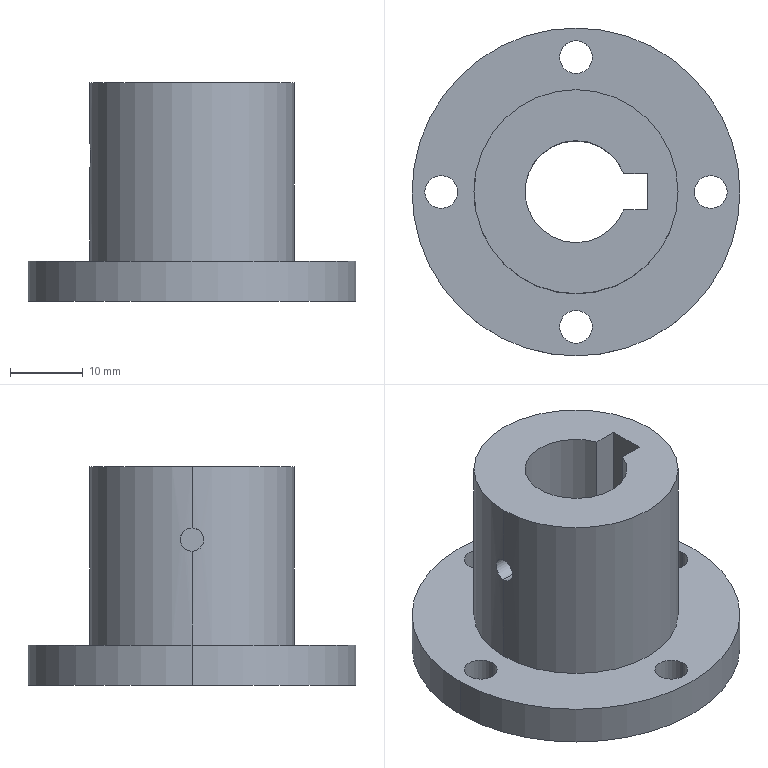Part | STEP file | Coupling | 1 solid | 21 faces | box 45 x 45 x 30 mm | volume 18366 mm3 | cylinder 15 | plane 6 | commonest cylinder face diameters 4.5 x8 3.2 x2 28 x2 45 x2 14 x1
STEP:
#1=CARTESIAN_POINT('',(-14.,0.,21.6));
#2=VERTEX_POINT('',#1);
#3=CARTESIAN_POINT('',(-14.,0.,18.4));
#4=VERTEX_POINT('',#3);
#5=CARTESIAN_POINT('',(-14.,0.,21.6));
#6=CARTESIAN_POINT('',(-14.,-0.1058,21.6));
#7=CARTESIAN_POINT('',(-13.999,-0.2098,21.59));
#8=CARTESIAN_POINT('',(-13.994,-0.4145,21.549));
#9=CARTESIAN_POINT('',(-13.991,-0.5161,21.518));
#10=CARTESIAN_POINT('',(-13.982,-0.7099,21.438));
#11=CARTESIAN_POINT('',(-13.977,-0.8017,21.389));
#12=CARTESIAN_POINT('',(-13.966,-0.9756,21.272));
#13=CARTESIAN_POINT('',(-13.96,-1.058,21.205));
#14=CARTESIAN_POINT('',(-13.942,-1.279,20.984));
#15=CARTESIAN_POINT('',(-13.93,-1.398,20.805));
#16=CARTESIAN_POINT('',(-13.913,-1.558,20.42));
#17=CARTESIAN_POINT('',(-13.908,-1.6,20.209));
#18=CARTESIAN_POINT('',(-13.908,-1.6,19.896));
#19=CARTESIAN_POINT('',(-13.909,-1.59,19.79));
#20=CARTESIAN_POINT('',(-13.914,-1.549,19.585));
#21=CARTESIAN_POINT('',(-13.917,-1.518,19.485));
#22=CARTESIAN_POINT('',(-13.926,-1.438,19.291));
#23=CARTESIAN_POINT('',(-13.931,-1.388,19.198));
#24=CARTESIAN_POINT('',(-13.942,-1.272,19.024));
#25=CARTESIAN_POINT('',(-13.948,-1.206,18.943));
#26=CARTESIAN_POINT('',(-13.96,-1.057,18.794));
#27=CARTESIAN_POINT('',(-13.966,-0.9761,18.728));
#28=CARTESIAN_POINT('',(-13.977,-0.8029,18.612));
#29=CARTESIAN_POINT('',(-13.982,-0.7093,18.562));
#30=CARTESIAN_POINT('',(-13.991,-0.5155,18.482));
#31=CARTESIAN_POINT('',(-13.994,-0.4158,18.451));
#32=CARTESIAN_POINT('',(-13.999,-0.2106,18.41));
#33=CARTESIAN_POINT('',(-14.,-0.1045,18.4));
#34=CARTESIAN_POINT('',(-14.,0.,18.4));
#35=B_SPLINE_CURVE_WITH_KNOTS('',3,(#5,#6,#7,#8,#9,#10,#11,#12,#13,#14,#15,#16,#17,#18,#19,#20,#21,#22,#23,#24,#25,#26,#27,#28,#29,#30,#31,#32,#33,#34),.UNSPECIFIED.,.F.,.F.,(4,2,2,2,2,2,2,2,2,2,2,2,2,2,4),(0.,0.0003129,0.0006258,0.0009387,0.001252,0.001877,0.002503,0.002816,0.003129,0.003442,0.003755,0.004068,0.004381,0.004694,0.005006),.UNSPECIFIED.);
#36=EDGE_CURVE('',#2,#4,#35,.T.);
#37=ORIENTED_EDGE('',*,*,#36,.F.);
#38=CARTESIAN_POINT('',(-7.,0.,21.6));
#39=VERTEX_POINT('',#38);
#40=CARTESIAN_POINT('',(-20.,0.,21.6));
#41=DIRECTION('',(1.,0.,0.));
#42=VECTOR('',#41,1000.);
#43=LINE('',#40,#42);
#44=EDGE_CURVE('',#2,#39,#43,.T.);
#45=ORIENTED_EDGE('',*,*,#44,.T.);
#46=CARTESIAN_POINT('',(-7.,0.,18.4));
#47=VERTEX_POINT('',#46);
#48=CARTESIAN_POINT('',(-7.,0.,18.4));
#49=CARTESIAN_POINT('',(-7.,-0.1061,18.4));
#50=CARTESIAN_POINT('',(-6.998,-0.2103,18.41));
#51=CARTESIAN_POINT('',(-6.988,-0.4153,18.451));
#52=CARTESIAN_POINT('',(-6.982,-0.5172,18.482));
#53=CARTESIAN_POINT('',(-6.964,-0.7108,18.563));
#54=CARTESIAN_POINT('',(-6.954,-0.8026,18.612));
#55=CARTESIAN_POINT('',(-6.932,-0.9762,18.728));
#56=CARTESIAN_POINT('',(-6.92,-1.058,18.795));
#57=CARTESIAN_POINT('',(-6.884,-1.279,19.016));
#58=CARTESIAN_POINT('',(-6.86,-1.398,19.194));
#59=CARTESIAN_POINT('',(-6.825,-1.558,19.579));
#60=CARTESIAN_POINT('',(-6.815,-1.6,19.79));
#61=CARTESIAN_POINT('',(-6.815,-1.6,20.104));
#62=CARTESIAN_POINT('',(-6.817,-1.59,20.211));
#63=CARTESIAN_POINT('',(-6.827,-1.549,20.416));
#64=CARTESIAN_POINT('',(-6.834,-1.518,20.516));
#65=CARTESIAN_POINT('',(-6.86,-1.397,20.807));
#66=CARTESIAN_POINT('',(-6.884,-1.28,20.983));
#67=CARTESIAN_POINT('',(-6.92,-1.057,21.206));
#68=CARTESIAN_POINT('',(-6.932,-0.9765,21.272));
#69=CARTESIAN_POINT('',(-6.954,-0.8035,21.388));
#70=CARTESIAN_POINT('',(-6.965,-0.7098,21.438));
#71=CARTESIAN_POINT('',(-6.982,-0.5165,21.518));
#72=CARTESIAN_POINT('',(-6.988,-0.4167,21.548));
#73=CARTESIAN_POINT('',(-6.998,-0.2108,21.59));
#74=CARTESIAN_POINT('',(-7.,-0.1046,21.6));
#75=CARTESIAN_POINT('',(-7.,0.,21.6));
#76=B_SPLINE_CURVE_WITH_KNOTS('',3,(#48,#49,#50,#51,#52,#53,#54,#55,#56,#57,#58,#59,#60,#61,#62,#63,#64,#65,#66,#67,#68,#69,#70,#71,#72,#73,#74,#75),.UNSPECIFIED.,.F.,.F.,(4,2,2,2,2,2,2,2,2,2,2,2,2,4),(0.,0.0003137,0.0006274,0.0009411,0.001255,0.001882,0.002509,0.002823,0.003137,0.003764,0.004078,0.004392,0.004705,0.005019),.UNSPECIFIED.);
#77=EDGE_CURVE('',#47,#39,#76,.T.);
#78=ORIENTED_EDGE('',*,*,#77,.F.);
#79=CARTESIAN_POINT('',(-20.,0.,18.4));
#80=DIRECTION('',(1.,0.,0.));
#81=VECTOR('',#80,1000.);
#82=LINE('',#79,#81);
#83=EDGE_CURVE('',#4,#47,#82,.T.);
#84=ORIENTED_EDGE('',*,*,#83,.F.);
#85=EDGE_LOOP('',(#37,#45,#78,#84));
#86=FACE_OUTER_BOUND('',#85,.T.);
#87=CARTESIAN_POINT('',(-20.,0.,20.));
#88=DIRECTION('',(1.,0.,0.));
#89=DIRECTION('',(0.,0.,-1.));
#90=AXIS2_PLACEMENT_3D('',#87,#88,#89);
#91=CYLINDRICAL_SURFACE('',#90,1.6);
#92=ADVANCED_FACE('',(#86),#91,.F.);
#93=CARTESIAN_POINT('',(-20.75,0.,0.));
#94=VERTEX_POINT('',#93);
#95=CARTESIAN_POINT('',(-16.25,0.,0.));
#96=VERTEX_POINT('',#95);
#97=CARTESIAN_POINT('',(-18.5,0.,0.));
#98=DIRECTION('',(0.,0.,1.));
#99=DIRECTION('',(1.,0.,0.));
#100=AXIS2_PLACEMENT_3D('',#97,#98,#99);
#101=CIRCLE('',#100,2.25);
#102=EDGE_CURVE('',#94,#96,#101,.T.);
#103=ORIENTED_EDGE('',*,*,#102,.F.);
#104=CARTESIAN_POINT('',(-20.75,0.,5.5));
#105=VERTEX_POINT('',#104);
#106=CARTESIAN_POINT('',(-20.75,0.,-34.5));
#107=DIRECTION('',(0.,0.,1.));
#108=VECTOR('',#107,1000.);
#109=LINE('',#106,#108);
#110=EDGE_CURVE('',#94,#105,#109,.T.);
#111=ORIENTED_EDGE('',*,*,#110,.T.);
#112=CARTESIAN_POINT('',(-16.25,0.,5.5));
#113=VERTEX_POINT('',#112);
#114=CARTESIAN_POINT('',(-18.5,0.,5.5));
#115=DIRECTION('',(0.,0.,1.));
#116=DIRECTION('',(-1.,0.,0.));
#117=AXIS2_PLACEMENT_3D('',#114,#115,#116);
#118=CIRCLE('',#117,2.25);
#119=EDGE_CURVE('',#105,#113,#118,.T.);
#120=ORIENTED_EDGE('',*,*,#119,.T.);
#121=CARTESIAN_POINT('',(-16.25,0.,-34.5));
#122=DIRECTION('',(0.,0.,1.));
#123=VECTOR('',#122,1000.);
#124=LINE('',#121,#123);
#125=EDGE_CURVE('',#96,#113,#124,.T.);
#126=ORIENTED_EDGE('',*,*,#125,.F.);
#127=EDGE_LOOP('',(#103,#111,#120,#126));
#128=FACE_OUTER_BOUND('',#127,.T.);
#129=CARTESIAN_POINT('',(-18.5,0.,-34.5));
#130=DIRECTION('',(0.,0.,1.));
#131=DIRECTION('',(1.,0.,0.));
#132=AXIS2_PLACEMENT_3D('',#129,#130,#131);
#133=CYLINDRICAL_SURFACE('',#132,2.25);
#134=ADVANCED_FACE('',(#128),#133,.F.);
#135=CARTESIAN_POINT('',(-2.25,18.5,0.));
#136=VERTEX_POINT('',#135);
#137=CARTESIAN_POINT('',(2.25,18.5,0.));
#138=VERTEX_POINT('',#137);
#139=CARTESIAN_POINT('',(0.,18.5,0.));
#140=DIRECTION('',(0.,0.,1.));
#141=DIRECTION('',(1.,0.,0.));
#142=AXIS2_PLACEMENT_3D('',#139,#140,#141);
#143=CIRCLE('',#142,2.25);
#144=EDGE_CURVE('',#136,#138,#143,.T.);
#145=ORIENTED_EDGE('',*,*,#144,.F.);
#146=CARTESIAN_POINT('',(-2.25,18.5,5.5));
#147=VERTEX_POINT('',#146);
#148=CARTESIAN_POINT('',(-2.25,18.5,-34.5));
#149=DIRECTION('',(0.,0.,1.));
#150=VECTOR('',#149,1000.);
#151=LINE('',#148,#150);
#152=EDGE_CURVE('',#136,#147,#151,.T.);
#153=ORIENTED_EDGE('',*,*,#152,.T.);
#154=CARTESIAN_POINT('',(2.25,18.5,5.5));
#155=VERTEX_POINT('',#154);
#156=CARTESIAN_POINT('',(0.,18.5,5.5));
#157=DIRECTION('',(0.,0.,1.));
#158=DIRECTION('',(0.,1.,0.));
#159=AXIS2_PLACEMENT_3D('',#156,#157,#158);
#160=CIRCLE('',#159,2.25);
#161=EDGE_CURVE('',#147,#155,#160,.T.);
#162=ORIENTED_EDGE('',*,*,#161,.T.);
#163=CARTESIAN_POINT('',(2.25,18.5,-34.5));
#164=DIRECTION('',(0.,0.,1.));
#165=VECTOR('',#164,1000.);
#166=LINE('',#163,#165);
#167=EDGE_CURVE('',#138,#155,#166,.T.);
#168=ORIENTED_EDGE('',*,*,#167,.F.);
#169=EDGE_LOOP('',(#145,#153,#162,#168));
#170=FACE_OUTER_BOUND('',#169,.T.);
#171=CARTESIAN_POINT('',(0.,18.5,-34.5));
#172=DIRECTION('',(0.,0.,1.));
#173=DIRECTION('',(1.,0.,0.));
#174=AXIS2_PLACEMENT_3D('',#171,#172,#173);
#175=CYLINDRICAL_SURFACE('',#174,2.25);
#176=ADVANCED_FACE('',(#170),#175,.F.);
#177=CARTESIAN_POINT('',(-2.25,-18.5,0.));
#178=VERTEX_POINT('',#177);
#179=CARTESIAN_POINT('',(2.25,-18.5,0.));
#180=VERTEX_POINT('',#179);
#181=CARTESIAN_POINT('',(0.,-18.5,0.));
#182=DIRECTION('',(0.,0.,1.));
#183=DIRECTION('',(1.,0.,0.));
#184=AXIS2_PLACEMENT_3D('',#181,#182,#183);
#185=CIRCLE('',#184,2.25);
#186=EDGE_CURVE('',#178,#180,#185,.T.);
#187=ORIENTED_EDGE('',*,*,#186,.F.);
#188=CARTESIAN_POINT('',(-2.25,-18.5,5.5));
#189=VERTEX_POINT('',#188);
#190=CARTESIAN_POINT('',(-2.25,-18.5,-34.5));
#191=DIRECTION('',(0.,0.,1.));
#192=VECTOR('',#191,1000.);
#193=LINE('',#190,#192);
#194=EDGE_CURVE('',#178,#189,#193,.T.);
#195=ORIENTED_EDGE('',*,*,#194,.T.);
#196=CARTESIAN_POINT('',(2.25,-18.5,5.5));
#197=VERTEX_POINT('',#196);
#198=CARTESIAN_POINT('',(0.,-18.5,5.5));
#199=DIRECTION('',(0.,0.,1.));
#200=DIRECTION('',(0.,-1.,0.));
#201=AXIS2_PLACEMENT_3D('',#198,#199,#200);
#202=CIRCLE('',#201,2.25);
#203=EDGE_CURVE('',#189,#197,#202,.T.);
#204=ORIENTED_EDGE('',*,*,#203,.T.);
#205=CARTESIAN_POINT('',(2.25,-18.5,-34.5));
#206=DIRECTION('',(0.,0.,1.));
#207=VECTOR('',#206,1000.);
#208=LINE('',#205,#207);
#209=EDGE_CURVE('',#180,#197,#208,.T.);
#210=ORIENTED_EDGE('',*,*,#209,.F.);
#211=EDGE_LOOP('',(#187,#195,#204,#210));
#212=FACE_OUTER_BOUND('',#211,.T.);
#213=CARTESIAN_POINT('',(0.,-18.5,-34.5));
#214=DIRECTION('',(0.,0.,1.));
#215=DIRECTION('',(1.,0.,0.));
#216=AXIS2_PLACEMENT_3D('',#213,#214,#215);
#217=CYLINDRICAL_SURFACE('',#216,2.25);
#218=ADVANCED_FACE('',(#212),#217,.F.);
#219=CARTESIAN_POINT('',(16.25,0.,0.));
#220=VERTEX_POINT('',#219);
#221=CARTESIAN_POINT('',(20.75,0.,0.));
#222=VERTEX_POINT('',#221);
#223=CARTESIAN_POINT('',(18.5,0.,0.));
#224=DIRECTION('',(0.,0.,1.));
#225=DIRECTION('',(1.,0.,0.));
#226=AXIS2_PLACEMENT_3D('',#223,#224,#225);
#227=CIRCLE('',#226,2.25);
#228=EDGE_CURVE('',#220,#222,#227,.T.);
#229=ORIENTED_EDGE('',*,*,#228,.F.);
#230=CARTESIAN_POINT('',(16.25,0.,5.5));
#231=VERTEX_POINT('',#230);
#232=CARTESIAN_POINT('',(16.25,0.,-34.5));
#233=DIRECTION('',(0.,0.,1.));
#234=VECTOR('',#233,1000.);
#235=LINE('',#232,#234);
#236=EDGE_CURVE('',#220,#231,#235,.T.);
#237=ORIENTED_EDGE('',*,*,#236,.T.);
#238=CARTESIAN_POINT('',(20.75,0.,5.5));
#239=VERTEX_POINT('',#238);
#240=CARTESIAN_POINT('',(18.5,0.,5.5));
#241=DIRECTION('',(0.,0.,1.));
#242=DIRECTION('',(1.,0.,0.));
#243=AXIS2_PLACEMENT_3D('',#240,#241,#242);
#244=CIRCLE('',#243,2.25);
#245=EDGE_CURVE('',#231,#239,#244,.T.);
#246=ORIENTED_EDGE('',*,*,#245,.T.);
#247=CARTESIAN_POINT('',(20.75,0.,-34.5));
#248=DIRECTION('',(0.,0.,1.));
#249=VECTOR('',#248,1000.);
#250=LINE('',#247,#249);
#251=EDGE_CURVE('',#222,#239,#250,.T.);
#252=ORIENTED_EDGE('',*,*,#251,.F.);
#253=EDGE_LOOP('',(#229,#237,#246,#252));
#254=FACE_OUTER_BOUND('',#253,.T.);
#255=CARTESIAN_POINT('',(18.5,0.,-34.5));
#256=DIRECTION('',(0.,0.,1.));
#257=DIRECTION('',(1.,0.,0.));
#258=AXIS2_PLACEMENT_3D('',#255,#256,#257);
#259=CYLINDRICAL_SURFACE('',#258,2.25);
#260=ADVANCED_FACE('',(#254),#259,.F.);
#261=CARTESIAN_POINT('',(-22.5,0.,5.5));
#262=VERTEX_POINT('',#261);
#263=CARTESIAN_POINT('',(22.5,0.,5.5));
#264=VERTEX_POINT('',#263);
#265=CARTESIAN_POINT('',(0.,0.,5.5));
#266=DIRECTION('',(0.,0.,-1.));
#267=DIRECTION('',(-1.,0.,0.));
#268=AXIS2_PLACEMENT_3D('',#265,#266,#267);
#269=CIRCLE('',#268,22.5);
#270=EDGE_CURVE('',#262,#264,#269,.T.);
#271=ORIENTED_EDGE('',*,*,#270,.T.);
#272=CARTESIAN_POINT('',(22.5,0.,0.));
#273=VERTEX_POINT('',#272);
#274=CARTESIAN_POINT('',(22.5,0.,5.5));
#275=DIRECTION('',(0.,0.,-1.));
#276=VECTOR('',#275,1000.);
#277=LINE('',#274,#276);
#278=EDGE_CURVE('',#264,#273,#277,.T.);
#279=ORIENTED_EDGE('',*,*,#278,.T.);
#280=CARTESIAN_POINT('',(-22.5,0.,0.));
#281=VERTEX_POINT('',#280);
#282=CARTESIAN_POINT('',(0.,0.,0.));
#283=DIRECTION('',(0.,0.,-1.));
#284=DIRECTION('',(-1.,0.,0.));
#285=AXIS2_PLACEMENT_3D('',#282,#283,#284);
#286=CIRCLE('',#285,22.5);
#287=EDGE_CURVE('',#281,#273,#286,.T.);
#288=ORIENTED_EDGE('',*,*,#287,.F.);
#289=CARTESIAN_POINT('',(-22.5,0.,5.5));
#290=DIRECTION('',(0.,0.,-1.));
#291=VECTOR('',#290,1000.);
#292=LINE('',#289,#291);
#293=EDGE_CURVE('',#262,#281,#292,.T.);
#294=ORIENTED_EDGE('',*,*,#293,.F.);
#295=EDGE_LOOP('',(#271,#279,#288,#294));
#296=FACE_OUTER_BOUND('',#295,.T.);
#297=CARTESIAN_POINT('',(0.,0.,5.5));
#298=DIRECTION('',(0.,0.,-1.));
#299=DIRECTION('',(-1.,0.,0.));
#300=AXIS2_PLACEMENT_3D('',#297,#298,#299);
#301=CYLINDRICAL_SURFACE('',#300,22.5);
#302=ADVANCED_FACE('',(#296),#301,.T.);
#303=CARTESIAN_POINT('',(14.,0.,30.));
#304=VERTEX_POINT('',#303);
#305=CARTESIAN_POINT('',(-14.,0.,30.));
#306=VERTEX_POINT('',#305);
#307=CARTESIAN_POINT('',(0.,0.,30.));
#308=DIRECTION('',(0.,0.,1.));
#309=DIRECTION('',(1.,0.,0.));
#310=AXIS2_PLACEMENT_3D('',#307,#308,#309);
#311=CIRCLE('',#310,14.);
#312=EDGE_CURVE('',#304,#306,#311,.T.);
#313=ORIENTED_EDGE('',*,*,#312,.F.);
#314=CARTESIAN_POINT('',(14.,0.,5.5));
#315=VERTEX_POINT('',#314);
#316=CARTESIAN_POINT('',(14.,0.,30.));
#317=DIRECTION('',(0.,0.,-1.));
#318=VECTOR('',#317,1000.);
#319=LINE('',#316,#318);
#320=EDGE_CURVE('',#304,#315,#319,.T.);
#321=ORIENTED_EDGE('',*,*,#320,.T.);
#322=CARTESIAN_POINT('',(-14.,0.,5.5));
#323=VERTEX_POINT('',#322);
#324=CARTESIAN_POINT('',(0.,0.,5.5));
#325=DIRECTION('',(0.,0.,-1.));
#326=DIRECTION('',(-1.,0.,0.));
#327=AXIS2_PLACEMENT_3D('',#324,#325,#326);
#328=CIRCLE('',#327,14.);
#329=EDGE_CURVE('',#323,#315,#328,.T.);
#330=ORIENTED_EDGE('',*,*,#329,.F.);
#331=CARTESIAN_POINT('',(-14.,0.,30.));
#332=DIRECTION('',(0.,0.,-1.));
#333=VECTOR('',#332,1000.);
#334=LINE('',#331,#333);
#335=EDGE_CURVE('',#4,#323,#334,.T.);
#336=ORIENTED_EDGE('',*,*,#335,.F.);
#337=CARTESIAN_POINT('',(-14.,0.,18.4));
#338=CARTESIAN_POINT('',(-14.,0.2089,18.4));
#339=CARTESIAN_POINT('',(-13.995,0.4195,18.442));
#340=CARTESIAN_POINT('',(-13.978,0.8046,18.601));
#341=CARTESIAN_POINT('',(-13.966,0.983,18.72));
#342=CARTESIAN_POINT('',(-13.948,1.204,18.942));
#343=CARTESIAN_POINT('',(-13.942,1.272,19.024));
#344=CARTESIAN_POINT('',(-13.931,1.388,19.197));
#345=CARTESIAN_POINT('',(-13.926,1.437,19.289));
#346=CARTESIAN_POINT('',(-13.918,1.518,19.483));
#347=CARTESIAN_POINT('',(-13.914,1.549,19.585));
#348=CARTESIAN_POINT('',(-13.909,1.589,19.789));
#349=CARTESIAN_POINT('',(-13.908,1.6,19.893));
#350=CARTESIAN_POINT('',(-13.908,1.6,20.105));
#351=CARTESIAN_POINT('',(-13.909,1.59,20.209));
#352=CARTESIAN_POINT('',(-13.914,1.549,20.413));
#353=CARTESIAN_POINT('',(-13.917,1.519,20.515));
#354=CARTESIAN_POINT('',(-13.926,1.438,20.709));
#355=CARTESIAN_POINT('',(-13.931,1.389,20.801));
#356=CARTESIAN_POINT('',(-13.942,1.273,20.975));
#357=CARTESIAN_POINT('',(-13.948,1.206,21.057));
#358=CARTESIAN_POINT('',(-13.966,0.9848,21.278));
#359=CARTESIAN_POINT('',(-13.978,0.8066,21.397));
#360=CARTESIAN_POINT('',(-13.995,0.4218,21.557));
#361=CARTESIAN_POINT('',(-14.,0.2116,21.6));
#362=CARTESIAN_POINT('',(-14.,0.,21.6));
#363=B_SPLINE_CURVE_WITH_KNOTS('',3,(#337,#338,#339,#340,#341,#342,#343,#344,#345,#346,#347,#348,#349,#350,#351,#352,#353,#354,#355,#356,#357,#358,#359,#360,#361,#362),.UNSPECIFIED.,.F.,.F.,(4,2,2,2,2,2,2,2,2,2,2,2,4),(0.005006,0.005632,0.006258,0.006571,0.006883,0.007196,0.007509,0.007822,0.008135,0.008448,0.00876,0.009386,0.01001),.UNSPECIFIED.);
#364=EDGE_CURVE('',#4,#2,#363,.T.);
#365=ORIENTED_EDGE('',*,*,#364,.T.);
#366=CARTESIAN_POINT('',(-14.,0.,30.));
#367=DIRECTION('',(0.,0.,-1.));
#368=VECTOR('',#367,1000.);
#369=LINE('',#366,#368);
#370=EDGE_CURVE('',#306,#2,#369,.T.);
#371=ORIENTED_EDGE('',*,*,#370,.F.);
#372=EDGE_LOOP('',(#313,#321,#330,#336,#365,#371));
#373=FACE_OUTER_BOUND('',#372,.T.);
#374=CARTESIAN_POINT('',(0.,0.,30.));
#375=DIRECTION('',(0.,0.,-1.));
#376=DIRECTION('',(-1.,0.,0.));
#377=AXIS2_PLACEMENT_3D('',#374,#375,#376);
#378=CYLINDRICAL_SURFACE('',#377,14.);
#379=ADVANCED_FACE('',(#373),#378,.T.);
#380=ORIENTED_EDGE('',*,*,#320,.F.);
#381=CARTESIAN_POINT('',(0.,0.,30.));
#382=DIRECTION('',(0.,0.,1.));
#383=DIRECTION('',(1.,0.,0.));
#384=AXIS2_PLACEMENT_3D('',#381,#382,#383);
#385=CIRCLE('',#384,14.);
#386=EDGE_CURVE('',#306,#304,#385,.T.);
#387=ORIENTED_EDGE('',*,*,#386,.F.);
#388=ORIENTED_EDGE('',*,*,#370,.T.);
#389=ORIENTED_EDGE('',*,*,#36,.T.);
#390=ORIENTED_EDGE('',*,*,#335,.T.);
#391=CARTESIAN_POINT('',(0.,0.,5.5));
#392=DIRECTION('',(0.,0.,-1.));
#393=DIRECTION('',(-1.,0.,0.));
#394=AXIS2_PLACEMENT_3D('',#391,#392,#393);
#395=CIRCLE('',#394,14.);
#396=EDGE_CURVE('',#315,#323,#395,.T.);
#397=ORIENTED_EDGE('',*,*,#396,.F.);
#398=EDGE_LOOP('',(#380,#387,#388,#389,#390,#397));
#399=FACE_OUTER_BOUND('',#398,.T.);
#400=CARTESIAN_POINT('',(0.,0.,30.));
#401=DIRECTION('',(0.,0.,-1.));
#402=DIRECTION('',(-1.,0.,0.));
#403=AXIS2_PLACEMENT_3D('',#400,#401,#402);
#404=CYLINDRICAL_SURFACE('',#403,14.);
#405=ADVANCED_FACE('',(#399),#404,.T.);
#406=CARTESIAN_POINT('',(9.8,2.5,30.));
#407=VERTEX_POINT('',#406);
#408=CARTESIAN_POINT('',(6.538,2.5,30.));
#409=VERTEX_POINT('',#408);
#410=CARTESIAN_POINT('',(9.8,2.5,30.));
#411=DIRECTION('',(-1.,0.,0.));
#412=VECTOR('',#411,1000.);
#413=LINE('',#410,#412);
#414=EDGE_CURVE('',#407,#409,#413,.T.);
#415=ORIENTED_EDGE('',*,*,#414,.F.);
#416=CARTESIAN_POINT('',(9.8,-2.5,30.));
#417=VERTEX_POINT('',#416);
#418=CARTESIAN_POINT('',(9.8,2.5,30.));
#419=DIRECTION('',(0.,1.,0.));
#420=VECTOR('',#419,1000.);
#421=LINE('',#418,#420);
#422=EDGE_CURVE('',#417,#407,#421,.T.);
#423=ORIENTED_EDGE('',*,*,#422,.F.);
#424=CARTESIAN_POINT('',(6.538,-2.5,30.));
#425=VERTEX_POINT('',#424);
#426=CARTESIAN_POINT('',(9.8,-2.5,30.));
#427=DIRECTION('',(1.,0.,0.));
#428=VECTOR('',#427,1000.);
#429=LINE('',#426,#428);
#430=EDGE_CURVE('',#425,#417,#429,.T.);
#431=ORIENTED_EDGE('',*,*,#430,.F.);
#432=CARTESIAN_POINT('',(0.,0.,30.));
#433=DIRECTION('',(0.,0.,1.));
#434=DIRECTION('',(1.,0.,0.));
#435=AXIS2_PLACEMENT_3D('',#432,#433,#434);
#436=CIRCLE('',#435,7.);
#437=EDGE_CURVE('',#409,#425,#436,.T.);
#438=ORIENTED_EDGE('',*,*,#437,.F.);
#439=EDGE_LOOP('',(#415,#423,#431,#438));
#440=FACE_BOUND('',#439,.T.);
#441=ORIENTED_EDGE('',*,*,#386,.T.);
#442=ORIENTED_EDGE('',*,*,#312,.T.);
#443=EDGE_LOOP('',(#441,#442));
#444=FACE_OUTER_BOUND('',#443,.T.);
#445=CARTESIAN_POINT('',(0.,0.,30.));
#446=DIRECTION('',(0.,0.,1.));
#447=DIRECTION('',(1.,0.,0.));
#448=AXIS2_PLACEMENT_3D('',#445,#446,#447);
#449=PLANE('',#448);
#450=ADVANCED_FACE('',(#440,#444),#449,.T.);
#451=CARTESIAN_POINT('',(-18.5,0.,0.));
#452=DIRECTION('',(0.,0.,1.));
#453=DIRECTION('',(1.,0.,0.));
#454=AXIS2_PLACEMENT_3D('',#451,#452,#453);
#455=CIRCLE('',#454,2.25);
#456=EDGE_CURVE('',#96,#94,#455,.T.);
#457=ORIENTED_EDGE('',*,*,#456,.T.);
#458=ORIENTED_EDGE('',*,*,#102,.T.);
#459=EDGE_LOOP('',(#457,#458));
#460=FACE_BOUND('',#459,.T.);
#461=CARTESIAN_POINT('',(0.,18.5,0.));
#462=DIRECTION('',(0.,0.,1.));
#463=DIRECTION('',(1.,0.,0.));
#464=AXIS2_PLACEMENT_3D('',#461,#462,#463);
#465=CIRCLE('',#464,2.25);
#466=EDGE_CURVE('',#138,#136,#465,.T.);
#467=ORIENTED_EDGE('',*,*,#466,.T.);
#468=ORIENTED_EDGE('',*,*,#144,.T.);
#469=EDGE_LOOP('',(#467,#468));
#470=FACE_BOUND('',#469,.T.);
#471=CARTESIAN_POINT('',(0.,-18.5,0.));
#472=DIRECTION('',(0.,0.,1.));
#473=DIRECTION('',(1.,0.,0.));
#474=AXIS2_PLACEMENT_3D('',#471,#472,#473);
#475=CIRCLE('',#474,2.25);
#476=EDGE_CURVE('',#180,#178,#475,.T.);
#477=ORIENTED_EDGE('',*,*,#476,.T.);
#478=ORIENTED_EDGE('',*,*,#186,.T.);
#479=EDGE_LOOP('',(#477,#478));
#480=FACE_BOUND('',#479,.T.);
#481=CARTESIAN_POINT('',(18.5,0.,0.));
#482=DIRECTION('',(0.,0.,1.));
#483=DIRECTION('',(1.,0.,0.));
#484=AXIS2_PLACEMENT_3D('',#481,#482,#483);
#485=CIRCLE('',#484,2.25);
#486=EDGE_CURVE('',#222,#220,#485,.T.);
#487=ORIENTED_EDGE('',*,*,#486,.T.);
#488=ORIENTED_EDGE('',*,*,#228,.T.);
#489=EDGE_LOOP('',(#487,#488));
#490=FACE_BOUND('',#489,.T.);
#491=CARTESIAN_POINT('',(9.8,-2.5,0.));
#492=VERTEX_POINT('',#491);
#493=CARTESIAN_POINT('',(9.8,2.5,0.));
#494=VERTEX_POINT('',#493);
#495=CARTESIAN_POINT('',(9.8,0.,0.));
#496=DIRECTION('',(0.,1.,0.));
#497=VECTOR('',#496,1000.);
#498=LINE('',#495,#497);
#499=EDGE_CURVE('',#492,#494,#498,.T.);
#500=ORIENTED_EDGE('',*,*,#499,.T.);
#501=CARTESIAN_POINT('',(6.538,2.5,0.));
#502=VERTEX_POINT('',#501);
#503=CARTESIAN_POINT('',(0.,2.5,0.));
#504=DIRECTION('',(-1.,0.,0.));
#505=VECTOR('',#504,1000.);
#506=LINE('',#503,#505);
#507=EDGE_CURVE('',#494,#502,#506,.T.);
#508=ORIENTED_EDGE('',*,*,#507,.T.);
#509=CARTESIAN_POINT('',(6.538,-2.5,0.));
#510=VERTEX_POINT('',#509);
#511=CARTESIAN_POINT('',(0.,0.,0.));
#512=DIRECTION('',(0.,0.,1.));
#513=DIRECTION('',(1.,0.,0.));
#514=AXIS2_PLACEMENT_3D('',#511,#512,#513);
#515=CIRCLE('',#514,7.);
#516=EDGE_CURVE('',#502,#510,#515,.T.);
#517=ORIENTED_EDGE('',*,*,#516,.T.);
#518=CARTESIAN_POINT('',(0.,-2.5,0.));
#519=DIRECTION('',(1.,0.,0.));
#520=VECTOR('',#519,1000.);
#521=LINE('',#518,#520);
#522=EDGE_CURVE('',#510,#492,#521,.T.);
#523=ORIENTED_EDGE('',*,*,#522,.T.);
#524=EDGE_LOOP('',(#500,#508,#517,#523));
#525=FACE_BOUND('',#524,.T.);
#526=ORIENTED_EDGE('',*,*,#287,.T.);
#527=CARTESIAN_POINT('',(0.,0.,0.));
#528=DIRECTION('',(0.,0.,-1.));
#529=DIRECTION('',(-1.,0.,0.));
#530=AXIS2_PLACEMENT_3D('',#527,#528,#529);
#531=CIRCLE('',#530,22.5);
#532=EDGE_CURVE('',#273,#281,#531,.T.);
#533=ORIENTED_EDGE('',*,*,#532,.T.);
#534=EDGE_LOOP('',(#526,#533));
#535=FACE_OUTER_BOUND('',#534,.T.);
#536=CARTESIAN_POINT('',(0.,0.,0.));
#537=DIRECTION('',(0.,0.,1.));
#538=DIRECTION('',(1.,0.,0.));
#539=AXIS2_PLACEMENT_3D('',#536,#537,#538);
#540=PLANE('',#539);
#541=ADVANCED_FACE('',(#460,#470,#480,#490,#525,#535),#540,.F.);
#542=ORIENTED_EDGE('',*,*,#77,.T.);
#543=CARTESIAN_POINT('',(-7.,0.,21.6));
#544=CARTESIAN_POINT('',(-7.,0.2092,21.6));
#545=CARTESIAN_POINT('',(-6.99,0.4204,21.558));
#546=CARTESIAN_POINT('',(-6.965,0.7094,21.438));
#547=CARTESIAN_POINT('',(-6.954,0.8029,21.388));
#548=CARTESIAN_POINT('',(-6.932,0.9767,21.272));
#549=CARTESIAN_POINT('',(-6.92,1.057,21.206));
#550=CARTESIAN_POINT('',(-6.896,1.205,21.058));
#551=CARTESIAN_POINT('',(-6.884,1.272,20.976));
#552=CARTESIAN_POINT('',(-6.861,1.388,20.803));
#553=CARTESIAN_POINT('',(-6.851,1.437,20.712));
#554=CARTESIAN_POINT('',(-6.825,1.558,20.42));
#555=CARTESIAN_POINT('',(-6.815,1.6,20.212));
#556=CARTESIAN_POINT('',(-6.815,1.6,19.895));
#557=CARTESIAN_POINT('',(-6.817,1.59,19.791));
#558=CARTESIAN_POINT('',(-6.827,1.549,19.586));
#559=CARTESIAN_POINT('',(-6.834,1.518,19.484));
#560=CARTESIAN_POINT('',(-6.859,1.398,19.194));
#561=CARTESIAN_POINT('',(-6.884,1.279,19.016));
#562=CARTESIAN_POINT('',(-6.932,0.9852,18.722));
#563=CARTESIAN_POINT('',(-6.956,0.8075,18.603));
#564=CARTESIAN_POINT('',(-6.981,0.5188,18.483));
#565=CARTESIAN_POINT('',(-6.988,0.417,18.452));
#566=CARTESIAN_POINT('',(-6.998,0.2107,18.41));
#567=CARTESIAN_POINT('',(-7.,0.1061,18.4));
#568=CARTESIAN_POINT('',(-7.,0.,18.4));
#569=B_SPLINE_CURVE_WITH_KNOTS('',3,(#543,#544,#545,#546,#547,#548,#549,#550,#551,#552,#553,#554,#555,#556,#557,#558,#559,#560,#561,#562,#563,#564,#565,#566,#567,#568),.UNSPECIFIED.,.F.,.F.,(4,2,2,2,2,2,2,2,2,2,2,2,4),(0.005019,0.005646,0.00596,0.006273,0.006587,0.006901,0.007528,0.007841,0.008155,0.008782,0.009409,0.009723,0.01004),.UNSPECIFIED.);
#570=EDGE_CURVE('',#39,#47,#569,.T.);
#571=ORIENTED_EDGE('',*,*,#570,.T.);
#572=EDGE_LOOP('',(#542,#571));
#573=FACE_BOUND('',#572,.T.);
#574=ORIENTED_EDGE('',*,*,#516,.F.);
#575=CARTESIAN_POINT('',(6.538,2.5,-5.));
#576=DIRECTION('',(0.,0.,1.));
#577=VECTOR('',#576,1000.);
#578=LINE('',#575,#577);
#579=EDGE_CURVE('',#502,#409,#578,.T.);
#580=ORIENTED_EDGE('',*,*,#579,.T.);
#581=ORIENTED_EDGE('',*,*,#437,.T.);
#582=CARTESIAN_POINT('',(6.538,-2.5,-5.));
#583=DIRECTION('',(0.,0.,-1.));
#584=VECTOR('',#583,1000.);
#585=LINE('',#582,#584);
#586=EDGE_CURVE('',#425,#510,#585,.T.);
#587=ORIENTED_EDGE('',*,*,#586,.T.);
#588=EDGE_LOOP('',(#574,#580,#581,#587));
#589=FACE_OUTER_BOUND('',#588,.T.);
#590=CARTESIAN_POINT('',(0.,0.,-5.));
#591=DIRECTION('',(0.,0.,1.));
#592=DIRECTION('',(1.,0.,0.));
#593=AXIS2_PLACEMENT_3D('',#590,#591,#592);
#594=CYLINDRICAL_SURFACE('',#593,7.);
#595=ADVANCED_FACE('',(#573,#589),#594,.F.);
#596=CARTESIAN_POINT('',(-18.5,0.,5.5));
#597=DIRECTION('',(0.,0.,1.));
#598=DIRECTION('',(-1.,0.,0.));
#599=AXIS2_PLACEMENT_3D('',#596,#597,#598);
#600=CIRCLE('',#599,2.25);
#601=EDGE_CURVE('',#113,#105,#600,.T.);
#602=ORIENTED_EDGE('',*,*,#601,.F.);
#603=ORIENTED_EDGE('',*,*,#119,.F.);
#604=EDGE_LOOP('',(#602,#603));
#605=FACE_BOUND('',#604,.T.);
#606=CARTESIAN_POINT('',(0.,18.5,5.5));
#607=DIRECTION('',(0.,0.,1.));
#608=DIRECTION('',(0.,1.,0.));
#609=AXIS2_PLACEMENT_3D('',#606,#607,#608);
#610=CIRCLE('',#609,2.25);
#611=EDGE_CURVE('',#155,#147,#610,.T.);
#612=ORIENTED_EDGE('',*,*,#611,.F.);
#613=ORIENTED_EDGE('',*,*,#161,.F.);
#614=EDGE_LOOP('',(#612,#613));
#615=FACE_BOUND('',#614,.T.);
#616=CARTESIAN_POINT('',(0.,-18.5,5.5));
#617=DIRECTION('',(0.,0.,1.));
#618=DIRECTION('',(0.,-1.,0.));
#619=AXIS2_PLACEMENT_3D('',#616,#617,#618);
#620=CIRCLE('',#619,2.25);
#621=EDGE_CURVE('',#197,#189,#620,.T.);
#622=ORIENTED_EDGE('',*,*,#621,.F.);
#623=ORIENTED_EDGE('',*,*,#203,.F.);
#624=EDGE_LOOP('',(#622,#623));
#625=FACE_BOUND('',#624,.T.);
#626=CARTESIAN_POINT('',(18.5,0.,5.5));
#627=DIRECTION('',(0.,0.,1.));
#628=DIRECTION('',(1.,0.,0.));
#629=AXIS2_PLACEMENT_3D('',#626,#627,#628);
#630=CIRCLE('',#629,2.25);
#631=EDGE_CURVE('',#239,#231,#630,.T.);
#632=ORIENTED_EDGE('',*,*,#631,.F.);
#633=ORIENTED_EDGE('',*,*,#245,.F.);
#634=EDGE_LOOP('',(#632,#633));
#635=FACE_BOUND('',#634,.T.);
#636=ORIENTED_EDGE('',*,*,#270,.F.);
#637=CARTESIAN_POINT('',(0.,0.,5.5));
#638=DIRECTION('',(0.,0.,-1.));
#639=DIRECTION('',(-1.,0.,0.));
#640=AXIS2_PLACEMENT_3D('',#637,#638,#639);
#641=CIRCLE('',#640,22.5);
#642=EDGE_CURVE('',#264,#262,#641,.T.);
#643=ORIENTED_EDGE('',*,*,#642,.F.);
#644=EDGE_LOOP('',(#636,#643));
#645=FACE_OUTER_BOUND('',#644,.T.);
#646=ORIENTED_EDGE('',*,*,#329,.T.);
#647=ORIENTED_EDGE('',*,*,#396,.T.);
#648=EDGE_LOOP('',(#646,#647));
#649=FACE_BOUND('',#648,.T.);
#650=CARTESIAN_POINT('',(0.,0.,5.5));
#651=DIRECTION('',(0.,0.,-1.));
#652=DIRECTION('',(-1.,0.,0.));
#653=AXIS2_PLACEMENT_3D('',#650,#651,#652);
#654=PLANE('',#653);
#655=ADVANCED_FACE('',(#605,#615,#625,#635,#645,#649),#654,.F.);
#656=ORIENTED_EDGE('',*,*,#278,.F.);
#657=ORIENTED_EDGE('',*,*,#642,.T.);
#658=ORIENTED_EDGE('',*,*,#293,.T.);
#659=ORIENTED_EDGE('',*,*,#532,.F.);
#660=EDGE_LOOP('',(#656,#657,#658,#659));
#661=FACE_OUTER_BOUND('',#660,.T.);
#662=CARTESIAN_POINT('',(0.,0.,5.5));
#663=DIRECTION('',(0.,0.,-1.));
#664=DIRECTION('',(-1.,0.,0.));
#665=AXIS2_PLACEMENT_3D('',#662,#663,#664);
#666=CYLINDRICAL_SURFACE('',#665,22.5);
#667=ADVANCED_FACE('',(#661),#666,.T.);
#668=CARTESIAN_POINT('',(9.8,-2.5,-10.));
#669=DIRECTION('',(0.,0.,1.));
#670=VECTOR('',#669,1000.);
#671=LINE('',#668,#670);
#672=EDGE_CURVE('',#492,#417,#671,.T.);
#673=ORIENTED_EDGE('',*,*,#672,.T.);
#674=ORIENTED_EDGE('',*,*,#422,.T.);
#675=CARTESIAN_POINT('',(9.8,2.5,-10.));
#676=DIRECTION('',(0.,0.,1.));
#677=VECTOR('',#676,1000.);
#678=LINE('',#675,#677);
#679=EDGE_CURVE('',#494,#407,#678,.T.);
#680=ORIENTED_EDGE('',*,*,#679,.F.);
#681=ORIENTED_EDGE('',*,*,#499,.F.);
#682=EDGE_LOOP('',(#673,#674,#680,#681));
#683=FACE_OUTER_BOUND('',#682,.T.);
#684=CARTESIAN_POINT('',(9.8,2.5,-10.));
#685=DIRECTION('',(1.,0.,0.));
#686=DIRECTION('',(0.,1.,0.));
#687=AXIS2_PLACEMENT_3D('',#684,#685,#686);
#688=PLANE('',#687);
#689=ADVANCED_FACE('',(#683),#688,.F.);
#690=ORIENTED_EDGE('',*,*,#679,.T.);
#691=ORIENTED_EDGE('',*,*,#414,.T.);
#692=ORIENTED_EDGE('',*,*,#579,.F.);
#693=ORIENTED_EDGE('',*,*,#507,.F.);
#694=EDGE_LOOP('',(#690,#691,#692,#693));
#695=FACE_OUTER_BOUND('',#694,.T.);
#696=CARTESIAN_POINT('',(9.8,2.5,-10.));
#697=DIRECTION('',(0.,1.,0.));
#698=DIRECTION('',(-1.,0.,0.));
#699=AXIS2_PLACEMENT_3D('',#696,#697,#698);
#700=PLANE('',#699);
#701=ADVANCED_FACE('',(#695),#700,.F.);
#702=ORIENTED_EDGE('',*,*,#586,.F.);
#703=ORIENTED_EDGE('',*,*,#430,.T.);
#704=ORIENTED_EDGE('',*,*,#672,.F.);
#705=ORIENTED_EDGE('',*,*,#522,.F.);
#706=EDGE_LOOP('',(#702,#703,#704,#705));
#707=FACE_OUTER_BOUND('',#706,.T.);
#708=CARTESIAN_POINT('',(9.8,-2.5,-10.));
#709=DIRECTION('',(0.,-1.,0.));
#710=DIRECTION('',(0.,0.,-1.));
#711=AXIS2_PLACEMENT_3D('',#708,#709,#710);
#712=PLANE('',#711);
#713=ADVANCED_FACE('',(#707),#712,.F.);
#714=ORIENTED_EDGE('',*,*,#236,.F.);
#715=ORIENTED_EDGE('',*,*,#486,.F.);
#716=ORIENTED_EDGE('',*,*,#251,.T.);
#717=ORIENTED_EDGE('',*,*,#631,.T.);
#718=EDGE_LOOP('',(#714,#715,#716,#717));
#719=FACE_OUTER_BOUND('',#718,.T.);
#720=CARTESIAN_POINT('',(18.5,0.,-34.5));
#721=DIRECTION('',(0.,0.,1.));
#722=DIRECTION('',(1.,0.,0.));
#723=AXIS2_PLACEMENT_3D('',#720,#721,#722);
#724=CYLINDRICAL_SURFACE('',#723,2.25);
#725=ADVANCED_FACE('',(#719),#724,.F.);
#726=ORIENTED_EDGE('',*,*,#194,.F.);
#727=ORIENTED_EDGE('',*,*,#476,.F.);
#728=ORIENTED_EDGE('',*,*,#209,.T.);
#729=ORIENTED_EDGE('',*,*,#621,.T.);
#730=EDGE_LOOP('',(#726,#727,#728,#729));
#731=FACE_OUTER_BOUND('',#730,.T.);
#732=CARTESIAN_POINT('',(0.,-18.5,-34.5));
#733=DIRECTION('',(0.,0.,1.));
#734=DIRECTION('',(1.,0.,0.));
#735=AXIS2_PLACEMENT_3D('',#732,#733,#734);
#736=CYLINDRICAL_SURFACE('',#735,2.25);
#737=ADVANCED_FACE('',(#731),#736,.F.);
#738=ORIENTED_EDGE('',*,*,#152,.F.);
#739=ORIENTED_EDGE('',*,*,#466,.F.);
#740=ORIENTED_EDGE('',*,*,#167,.T.);
#741=ORIENTED_EDGE('',*,*,#611,.T.);
#742=EDGE_LOOP('',(#738,#739,#740,#741));
#743=FACE_OUTER_BOUND('',#742,.T.);
#744=CARTESIAN_POINT('',(0.,18.5,-34.5));
#745=DIRECTION('',(0.,0.,1.));
#746=DIRECTION('',(1.,0.,0.));
#747=AXIS2_PLACEMENT_3D('',#744,#745,#746);
#748=CYLINDRICAL_SURFACE('',#747,2.25);
#749=ADVANCED_FACE('',(#743),#748,.F.);
#750=ORIENTED_EDGE('',*,*,#110,.F.);
#751=ORIENTED_EDGE('',*,*,#456,.F.);
#752=ORIENTED_EDGE('',*,*,#125,.T.);
#753=ORIENTED_EDGE('',*,*,#601,.T.);
#754=EDGE_LOOP('',(#750,#751,#752,#753));
#755=FACE_OUTER_BOUND('',#754,.T.);
#756=CARTESIAN_POINT('',(-18.5,0.,-34.5));
#757=DIRECTION('',(0.,0.,1.));
#758=DIRECTION('',(1.,0.,0.));
#759=AXIS2_PLACEMENT_3D('',#756,#757,#758);
#760=CYLINDRICAL_SURFACE('',#759,2.25);
#761=ADVANCED_FACE('',(#755),#760,.F.);
#762=ORIENTED_EDGE('',*,*,#44,.F.);
#763=ORIENTED_EDGE('',*,*,#364,.F.);
#764=ORIENTED_EDGE('',*,*,#83,.T.);
#765=ORIENTED_EDGE('',*,*,#570,.F.);
#766=EDGE_LOOP('',(#762,#763,#764,#765));
#767=FACE_OUTER_BOUND('',#766,.T.);
#768=CARTESIAN_POINT('',(-20.,0.,20.));
#769=DIRECTION('',(1.,0.,0.));
#770=DIRECTION('',(0.,0.,-1.));
#771=AXIS2_PLACEMENT_3D('',#768,#769,#770);
#772=CYLINDRICAL_SURFACE('',#771,1.6);
#773=ADVANCED_FACE('',(#767),#772,.F.);
#774=CLOSED_SHELL('',(#92,#134,#176,#218,#260,#302,#379,#405,#450,#541,#595,#655,#667,#689,#701,#713,#725,#737,#749,#761,#773));
#775=MANIFOLD_SOLID_BREP('',#774);
#776=CARTESIAN_POINT('',(0.,0.,0.));
#777=DIRECTION('',(0.,0.,1.));
#778=DIRECTION('',(1.,0.,0.));
#779=AXIS2_PLACEMENT_3D('',#776,#777,#778);
#780=(LENGTH_UNIT()NAMED_UNIT(*)SI_UNIT(.MILLI.,.METRE.));
#781=UNCERTAINTY_MEASURE_WITH_UNIT(LENGTH_MEASURE(0.00001),#780,'','');
#782=(NAMED_UNIT(*)PLANE_ANGLE_UNIT()SI_UNIT($,.RADIAN.));
#783=(NAMED_UNIT(*)SI_UNIT($,.STERADIAN.)SOLID_ANGLE_UNIT());
#784=(GEOMETRIC_REPRESENTATION_CONTEXT(3)GLOBAL_UNCERTAINTY_ASSIGNED_CONTEXT((#781))GLOBAL_UNIT_ASSIGNED_CONTEXT((#780,#782,#783))REPRESENTATION_CONTEXT('',''));
#785=ADVANCED_BREP_SHAPE_REPRESENTATION('',(#775,#779),#784);